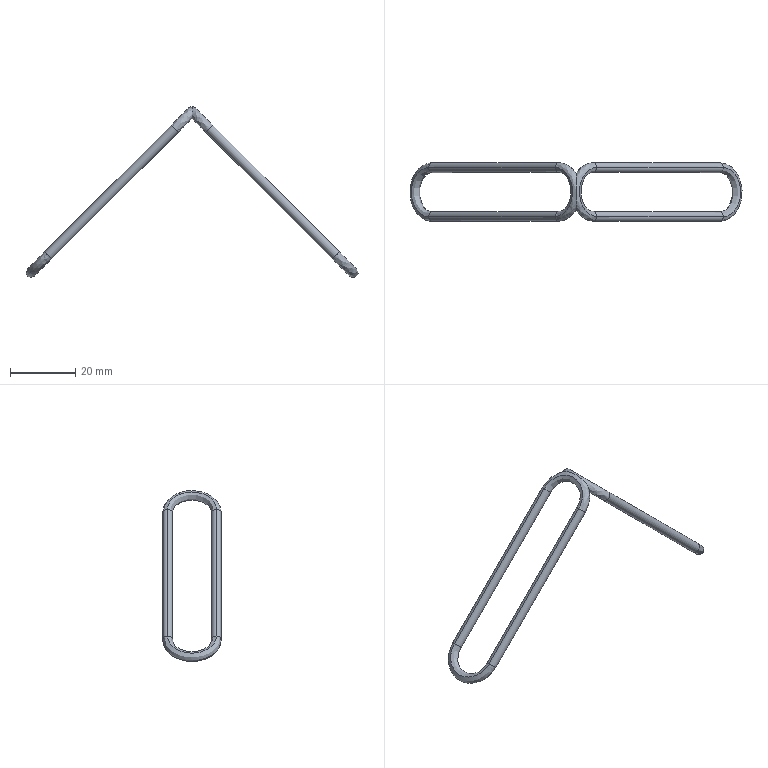Part | SolidWorks | features MirrorPattern 1, RefAxis 1, Sweep 1 | 1 solid | 16 faces | box 101.995 x 18 x 52.497 mm | volume 2170 mm3 | cylinder 8 | spline 8 | commonest cylinder face diameters 3 x8